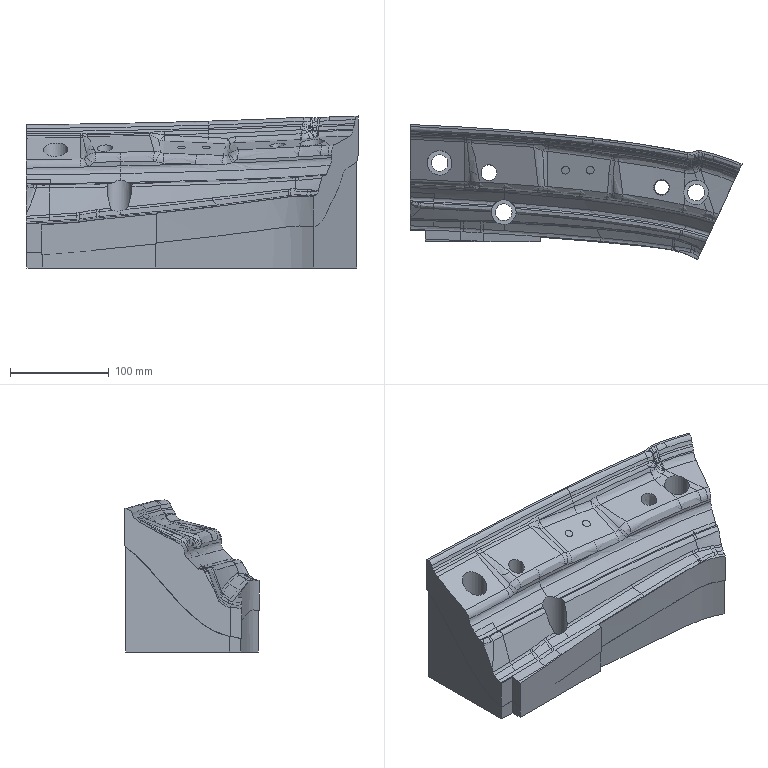Part | NX | features solid 2 | 1 solid | 233 faces | box 336.59 x 136.584 x 154.109 mm | volume 3398501 mm3 | spline 207 | plane 17 | cylinder 9 | commonest cylinder face diameters 25 x5 17 x3 16 x1